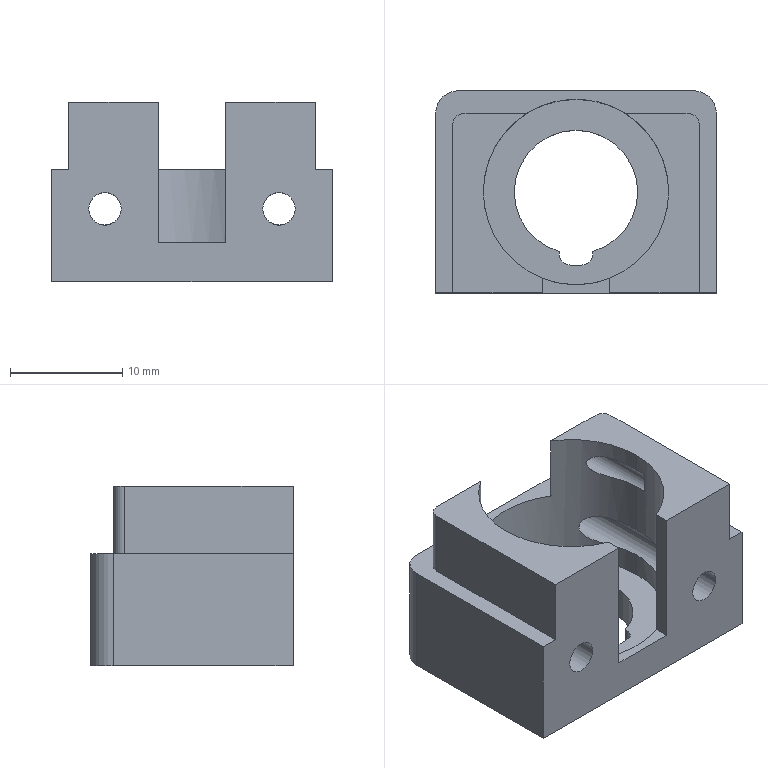Part | STEP file | ASND-0110-4216107200 | 1 solid | 44 faces | box 25 x 18 x 16 mm | volume 3261 mm3 | plane 21 | cylinder 19 | cone 4 | commonest cylinder face diameters 2 x4 2.05 x4 2.9 x4 11 x3 4 x2 16.5 x2